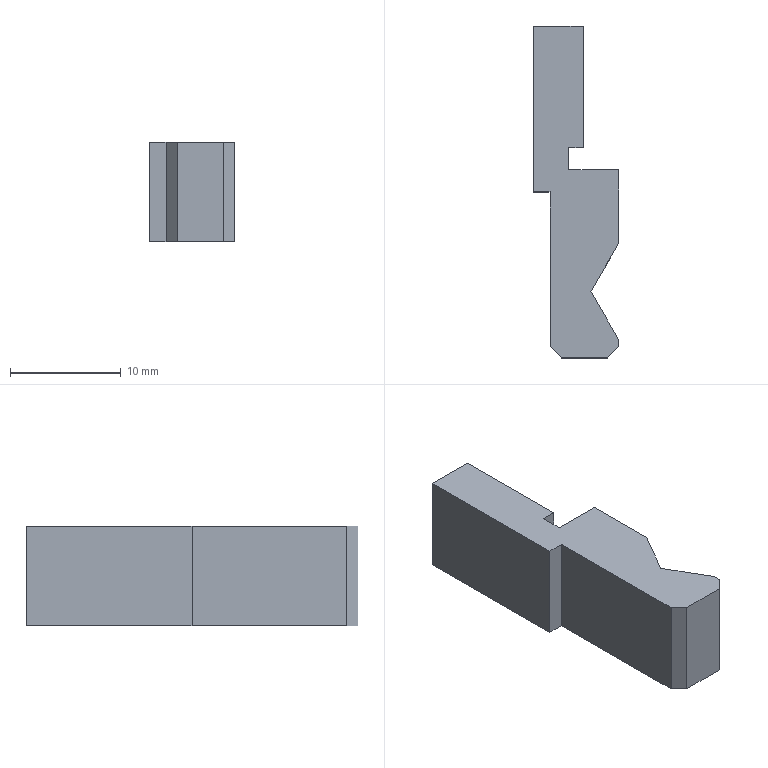Part | STEP file | 2012-06-08-011 | 1 solid | 23 faces | box 7.7 x 30 x 9 mm | volume 1306 mm3 | plane 23